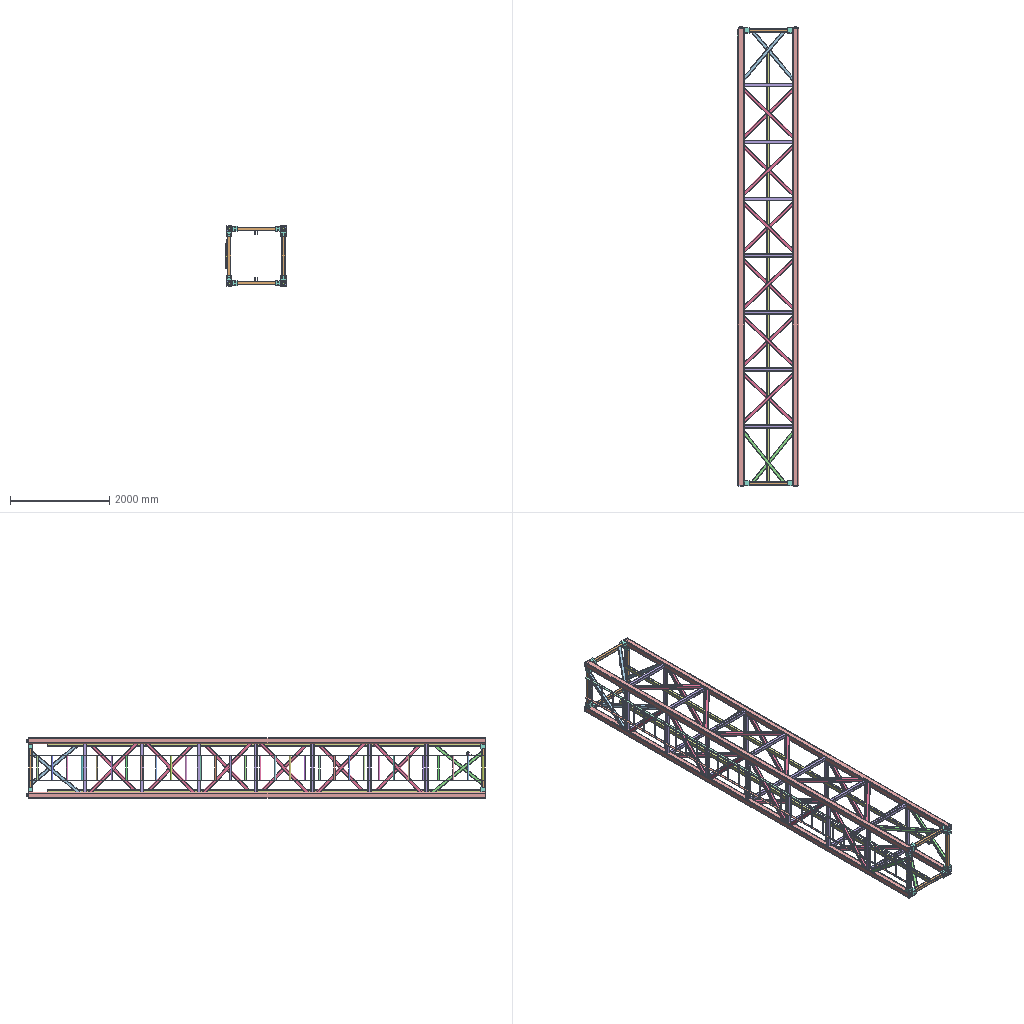Assembly | SolidWorks | 13 different items | 107 placed | box 1235 x 9290 x 1220 mm
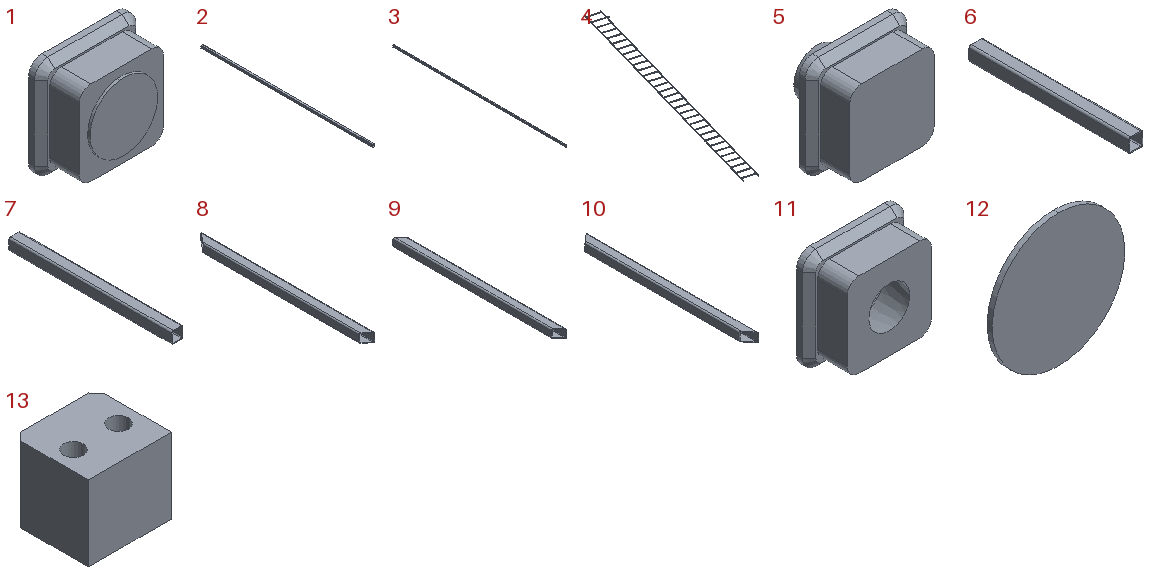Parts list (item | name | quantity | parent item | size | volume | features):
1 | (subassembly) | x4 | - | 120 x 53 x 120 mm | 407856 mm3 | -
2 | - | x4 | - | 120 x 9220 x 120 mm | 38826807 mm3 | features WeldMemberFeat 1, WeldmentFeature 1
3 | - | x2 | - | 60 x 8850 x 80 mm | 10935232 mm3 | features WeldMemberFeat 1, WeldmentFeature 1
4 | - | x1 | - | 3019 x 8991 x 40 mm | 7846988 mm3 | features WeldMemberFeat 2, Chamfer 1, LPattern 1, Sweep 1, WeldCornerFeat 1, WeldmentFeature 1
5 | - | x4 | - | 120 x 90 x 120 mm | 672208 mm3 | features Chamfer 2, ICE 2, Revolution 1
6 | - | x8 | - | 70 x 780 x 70 mm | 963783 mm3 | features WeldMemberFeat 1, WeldmentFeature 1
7 | - | x28 | - | 70 x 980 x 70 mm | 1210907 mm3 | features WeldMemberFeat 1, WeldmentFeature 1
8 | - | x4 | - | 70 x 1340 x 70 mm | 1567074 mm3 | features ICE 1, WeldMemberFeat 1, WeldmentFeature 1
9 | - | x24 | - | 70 x 1421 x 70 mm | 1672765 mm3 | features ICE 1, WeldMemberFeat 1, WeldmentFeature 1
10 | - | x4 | - | 70 x 1302 x 70 mm | 1520953 mm3 | features ICE 1, WeldMemberFeat 1, WeldmentFeature 1
11 | - | x4 | in 1 | 120 x 50 x 120 mm | 392776 mm3 | features Chamfer 1, Extrusion 1, ICE 1, RevCut 1
12 | - | x4 | in 1 | 80 x 3 x 80 mm | 15080 mm3 | features Extrusion 1
13 | - | x16 | - | 110 x 100 x 100 mm | 983814 mm3 | features Chamfer 1, Extrusion 1, HoleWzd 1
Mates (type | each side: item.copy, entity, surface, feature):
In the top assembly
Symmetric | 2.1 face plane Cold-formed hollow square steel (GB/T 6728-2002) 120×120×10(1) | 2.2 face plane Cold-formed hollow square steel (GB/T 6728-2002) 120×120×10(1) | assembly plane
DistanceDim | assembly plane | 2.1 face plane Cold-formed hollow square steel (GB/T 6728-2002) 120×120×10(1)
Coincident | 2.3 face plane Cold-formed hollow square steel (GB/T 6728-2002) 120×120×10(1) | assembly plane
Coincident | 2.1 face plane Cold-formed hollow square steel (GB/T 6728-2002) 120×120×10(1) | 11.1 face plane Boss-Extrude1
Width | 11.1 face plane Boss-Extrude2 | 11.1 face plane Boss-Extrude2 | 2.1 face plane Cold-formed hollow square steel (GB/T 6728-2002) 120×120×10(1) | 2.1 face plane Cold-formed hollow square steel (GB/T 6728-2002) 120×120×10(1)
Width | 2.1 face plane Cold-formed hollow square steel (GB/T 6728-2002) 120×120×10(1) | 2.1 face plane Cold-formed hollow square steel (GB/T 6728-2002) 120×120×10(1) | 11.1 face plane Boss-Extrude1 | 11.1 face plane Boss-Extrude1
Coincident | 2.1 face plane Cold-formed hollow square steel (GB/T 6728-2002) 120×120×10(1) | 5.1 face plane Boss-Extrude1
Width | 2.1 face plane Cold-formed hollow square steel (GB/T 6728-2002) 120×120×10(1) | 2.1 face plane Cold-formed hollow square steel (GB/T 6728-2002) 120×120×10(1) | 5.1 face plane Boss-Extrude1 | 5.1 face plane Boss-Extrude1 | 2 times
Coincident | 13.1 face plane Boss-Extrude1 | 11.2 face plane Boss-Extrude1
Width | 13.1 face plane Boss-Extrude1 | 13.1 face plane Boss-Extrude1 | 2.3 face plane Cold-formed hollow square steel (GB/T 6728-2002) 120×120×10(1) | 2.3 face plane Cold-formed hollow square steel (GB/T 6728-2002) 120×120×10(1)
Coincident | 13.1 face plane Boss-Extrude1 | 2.3 face plane Cold-formed hollow square steel (GB/T 6728-2002) 120×120×10(1)
Coincident | 2.3 face plane Cold-formed hollow square steel (GB/T 6728-2002) 120×120×10(1) | 13.2 face plane Boss-Extrude1
Coincident | 13.1 face plane Boss-Extrude1 | 13.2 face plane Boss-Extrude1
Width | 13.2 face plane Boss-Extrude1 | 13.2 face plane Boss-Extrude1 | 2.3 face plane Cold-formed hollow square steel (GB/T 6728-2002) 120×120×10(1) | 2.3 face plane Cold-formed hollow square steel (GB/T 6728-2002) 120×120×10(1)
Coincident | 13.3 face plane Boss-Extrude1 | 13.4 face plane Boss-Extrude1
Coincident | 13.1 face plane Boss-Extrude1 | 13.4 face plane Boss-Extrude1 | 2 times
Coincident | 13.2 face plane Boss-Extrude1 | 13.3 face plane Boss-Extrude1 | 2 times
Coincident | 5.2 face plane Boss-Extrude1 | 13.3 face plane Boss-Extrude1
Coincident | 6.1 face plane 19 (WeldMemberFeat) (+4 more in 5 files) Cold-formed hollow square steel (GB/T 6728-2002) 70×70×5(1) | 6.2 face plane 19 (WeldMemberFeat) (+4 more in 5 files) Cold-formed hollow square steel (GB/T 6728-2002) 70×70×5(1) | 2 times
Width | 6.2 face plane 19 (WeldMemberFeat) (+4 more in 5 files) Cold-formed hollow square steel (GB/T 6728-2002) 70×70×5(1) | 6.2 face plane 19 (WeldMemberFeat) (+4 more in 5 files) Cold-formed hollow square steel (GB/T 6728-2002) 70×70×5(1) | 13.5 face plane Boss-Extrude1 | 13.5 face plane Boss-Extrude1
Coincident | 13.1 face plane Boss-Extrude1 | 6.1 face plane 19 (WeldMemberFeat) (+4 more in 5 files) Cold-formed hollow square steel (GB/T 6728-2002) 70×70×5(1)
Width | 6.1 face plane 19 (WeldMemberFeat) (+4 more in 5 files) Cold-formed hollow square steel (GB/T 6728-2002) 70×70×5(1) | 6.1 face plane 19 (WeldMemberFeat) (+4 more in 5 files) Cold-formed hollow square steel (GB/T 6728-2002) 70×70×5(1) | 13.1 face plane Boss-Extrude1 | 13.1 face plane Boss-Extrude1
Width | 13.1 face plane Boss-Extrude1 | 13.1 face plane Boss-Extrude1 | 6.1 face plane 19 (WeldMemberFeat) (+4 more in 5 files) Cold-formed hollow square steel (GB/T 6728-2002) 70×70×5(1) | 6.1 face plane 19 (WeldMemberFeat) (+4 more in 5 files) Cold-formed hollow square steel (GB/T 6728-2002) 70×70×5(1)
Coincident | 6.3 face plane 19 (WeldMemberFeat) (+4 more in 5 files) Cold-formed hollow square steel (GB/T 6728-2002) 70×70×5(1) | 6.4 face plane 19 (WeldMemberFeat) (+4 more in 5 files) Cold-formed hollow square steel (GB/T 6728-2002) 70×70×5(1) | 2 times
Coincident | 13.2 face plane Boss-Extrude1 | 6.3 face plane 19 (WeldMemberFeat) (+4 more in 5 files) Cold-formed hollow square steel (GB/T 6728-2002) 70×70×5(1)
Width | 6.3 face plane 19 (WeldMemberFeat) (+4 more in 5 files) Cold-formed hollow square steel (GB/T 6728-2002) 70×70×5(1) | 6.3 face plane 19 (WeldMemberFeat) (+4 more in 5 files) Cold-formed hollow square steel (GB/T 6728-2002) 70×70×5(1) | 13.2 face plane Boss-Extrude1 | 13.2 face plane Boss-Extrude1 | 2 times
Width | 6.4 face plane 19 (WeldMemberFeat) (+4 more in 5 files) Cold-formed hollow square steel (GB/T 6728-2002) 70×70×5(1) | 6.4 face plane 19 (WeldMemberFeat) (+4 more in 5 files) Cold-formed hollow square steel (GB/T 6728-2002) 70×70×5(1) | 13.3 face plane Boss-Extrude1 | 13.3 face plane Boss-Extrude1
Width | 7.1 face plane 19 (WeldMemberFeat) (+4 more in 5 files) Cold-formed hollow square steel (GB/T 6728-2002) 70×70×5(1) | 7.1 face plane 19 (WeldMemberFeat) (+4 more in 5 files) Cold-formed hollow square steel (GB/T 6728-2002) 70×70×5(1) | 2.4 face plane Cold-formed hollow square steel (GB/T 6728-2002) 120×120×10(1) | 2.4 face plane Cold-formed hollow square steel (GB/T 6728-2002) 120×120×10(1)
Coincident | 7.1 face plane 19 (WeldMemberFeat) (+4 more in 5 files) Cold-formed hollow square steel (GB/T 6728-2002) 70×70×5(1) | 2.4 face plane Cold-formed hollow square steel (GB/T 6728-2002) 120×120×10(1)
DistanceDim | 11.2 face plane Boss-Extrude1 | 7.1 face plane 19 (WeldMemberFeat) (+4 more in 5 files) Cold-formed hollow square steel (GB/T 6728-2002) 70×70×5(1)
Coincident | 9.1 face plane Cut-Extrude1 | 2.4 face plane Cold-formed hollow square steel (GB/T 6728-2002) 120×120×10(1)
Coincident | 2.3 face plane Cold-formed hollow square steel (GB/T 6728-2002) 120×120×10(1) | 9.2 face plane Cut-Extrude1
DistanceDim | 9.2 edge | 7.2 face plane 19 (WeldMemberFeat) (+4 more in 5 files) Cold-formed hollow square steel (GB/T 6728-2002) 70×70×5(1)
Coincident | 2.1 face plane Cold-formed hollow square steel (GB/T 6728-2002) 120×120×10(1) | 9.3 face plane Cut-Extrude1
DistanceDim | 9.3 edge | 7.3 face plane 19 (WeldMemberFeat) (+4 more in 5 files) Cold-formed hollow square steel (GB/T 6728-2002) 70×70×5(1)
Coincident | 9.3 face plane 19 (WeldMemberFeat) (+4 more in 5 files) Cold-formed hollow square steel (GB/T 6728-2002) 70×70×5(1) | 9.4 face plane 19 (WeldMemberFeat) (+4 more in 5 files) Cold-formed hollow square steel (GB/T 6728-2002) 70×70×5(1)
Coincident | 2.2 face plane Cold-formed hollow square steel (GB/T 6728-2002) 120×120×10(1) | 9.4 face plane Cut-Extrude1
DistanceDim | 9.4 edge | 7.4 face plane 19 (WeldMemberFeat) (+4 more in 5 files) Cold-formed hollow square steel (GB/T 6728-2002) 70×70×5(1)
Coincident | 6.2 face plane 19 (WeldMemberFeat) (+4 more in 5 files) Cold-formed hollow square steel (GB/T 6728-2002) 70×70×5(1) | 10.1 face plane Cut-Extrude1
Coincident | 6.2 face plane 19 (WeldMemberFeat) (+4 more in 5 files) Cold-formed hollow square steel (GB/T 6728-2002) 70×70×5(1) | 10.1 face plane 19 (WeldMemberFeat) (+4 more in 5 files) Cold-formed hollow square steel (GB/T 6728-2002) 70×70×5(1)
Coincident | 2.3 face plane Cold-formed hollow square steel (GB/T 6728-2002) 120×120×10(1) | 10.1 face plane Cut-Extrude1
Coincident | 2.2 face plane Cold-formed hollow square steel (GB/T 6728-2002) 120×120×10(1) | 10.2 face plane Cut-Extrude1
Coincident | assembly face | 10.2 face plane 19 (WeldMemberFeat) (+4 more in 5 files) Cold-formed hollow square steel (GB/T 6728-2002) 70×70×5(1)
Coincident | 6.5 face plane 19 (WeldMemberFeat) (+4 more in 5 files) Cold-formed hollow square steel (GB/T 6728-2002) 70×70×5(1) | 10.2 face plane Cut-Extrude1
Coincident | 7.1 face plane 19 (WeldMemberFeat) (+4 more in 5 files) Cold-formed hollow square steel (GB/T 6728-2002) 70×70×5(1) | 7.5 face plane 19 (WeldMemberFeat) (+4 more in 5 files) Cold-formed hollow square steel (GB/T 6728-2002) 70×70×5(1)
Coincident | 2.3 face plane Cold-formed hollow square steel (GB/T 6728-2002) 120×120×10(1) | 7.5 face plane 19 (WeldMemberFeat) (+4 more in 5 files) Cold-formed hollow square steel (GB/T 6728-2002) 70×70×5(1)
Width | 7.5 face plane 19 (WeldMemberFeat) (+4 more in 5 files) Cold-formed hollow square steel (GB/T 6728-2002) 70×70×5(1) | 7.5 face plane 19 (WeldMemberFeat) (+4 more in 5 files) Cold-formed hollow square steel (GB/T 6728-2002) 70×70×5(1) | 2.3 face plane Cold-formed hollow square steel (GB/T 6728-2002) 120×120×10(1) | 2.3 face plane Cold-formed hollow square steel (GB/T 6728-2002) 120×120×10(1)
Coincident | 7.5 face plane 19 (WeldMemberFeat) (+4 more in 5 files) Cold-formed hollow square steel (GB/T 6728-2002) 70×70×5(1) | 7.6 face plane 19 (WeldMemberFeat) (+4 more in 5 files) Cold-formed hollow square steel (GB/T 6728-2002) 70×70×5(1) | 2 times
Width | 7.6 face plane 19 (WeldMemberFeat) (+4 more in 5 files) Cold-formed hollow square steel (GB/T 6728-2002) 70×70×5(1) | 7.6 face plane 19 (WeldMemberFeat) (+4 more in 5 files) Cold-formed hollow square steel (GB/T 6728-2002) 70×70×5(1) | 2.2 face plane Cold-formed hollow square steel (GB/T 6728-2002) 120×120×10(1) | 2.2 face plane Cold-formed hollow square steel (GB/T 6728-2002) 120×120×10(1)
Coincident | 4.1 face plane GB/T 704-1988 hot-rolled flat steel 40×6(1) | 6.4 face plane 19 (WeldMemberFeat) (+4 more in 5 files) Cold-formed hollow square steel (GB/T 6728-2002) 70×70×5(1)
Width | 2.3 face plane Cold-formed hollow square steel (GB/T 6728-2002) 120×120×10(1) | 2.1 face plane Cold-formed hollow square steel (GB/T 6728-2002) 120×120×10(1) | 4.1 face plane GB/T 704-1988 hot-rolled flat steel 40×6(1) | 4.1 face plane GB/T 704-1988 hot-rolled flat steel 40×6(1)
Coincident | 4.1 face plane GB/T 704-1988 hot-rolled flat steel 40×6(1) | 11.2 face plane Boss-Extrude1
Coincident | 6.2 face plane 19 (WeldMemberFeat) (+4 more in 5 files) Cold-formed hollow square steel (GB/T 6728-2002) 70×70×5(1) | 3.1 face plane Cold-formed hollow rectangular steel (GB/T 6728-2002) 80×60×5(1)
Coincident | 3.1 plane | assembly plane
Coincident | 8.1 face plane Cut-Extrude1 | 6.1 face plane 19 (WeldMemberFeat) (+4 more in 5 files) Cold-formed hollow square steel (GB/T 6728-2002) 70×70×5(1)
Coincident | 8.1 face plane Cut-Extrude1 | 2.4 face plane Cold-formed hollow square steel (GB/T 6728-2002) 120×120×10(1)
Coincident | 6.6 face plane 19 (WeldMemberFeat) (+4 more in 5 files) Cold-formed hollow square steel (GB/T 6728-2002) 70×70×5(1) | 8.2 face plane Cut-Extrude1
Coincident | 2.1 face plane Cold-formed hollow square steel (GB/T 6728-2002) 120×120×10(1) | 8.2 face plane Cut-Extrude1
Coincident | 6.3 face plane 19 (WeldMemberFeat) (+4 more in 5 files) Cold-formed hollow square steel (GB/T 6728-2002) 70×70×5(1) | 8.3 face plane Cut-Extrude1
Coincident | 2.3 face plane Cold-formed hollow square steel (GB/T 6728-2002) 120×120×10(1) | 8.3 face plane Cut-Extrude1
Coincident | 6.7 face plane 19 (WeldMemberFeat) (+4 more in 5 files) Cold-formed hollow square steel (GB/T 6728-2002) 70×70×5(1) | 8.4 face plane Cut-Extrude1
Coincident | 2.2 face plane Cold-formed hollow square steel (GB/T 6728-2002) 120×120×10(1) | 8.4 face plane Cut-Extrude1
Coincident | 2.1 face plane Cold-formed hollow square steel (GB/T 6728-2002) 120×120×10(1) | 10.3 face plane Cut-Extrude1
Coincident | assembly face | 10.3 face plane 19 (WeldMemberFeat) (+4 more in 5 files) Cold-formed hollow square steel (GB/T 6728-2002) 70×70×5(1)
Coincident | 6.4 face plane 19 (WeldMemberFeat) (+4 more in 5 files) Cold-formed hollow square steel (GB/T 6728-2002) 70×70×5(1) | 10.3 face plane Cut-Extrude1
Coincident | 6.8 face plane 19 (WeldMemberFeat) (+4 more in 5 files) Cold-formed hollow square steel (GB/T 6728-2002) 70×70×5(1) | 10.4 face plane Cut-Extrude1
Coincident | assembly face | 10.4 face plane 19 (WeldMemberFeat) (+4 more in 5 files) Cold-formed hollow square steel (GB/T 6728-2002) 70×70×5(1)
Coincident | 2.4 face plane Cold-formed hollow square steel (GB/T 6728-2002) 120×120×10(1) | 10.4 face plane Cut-Extrude1
Coincident | 2.1 face plane Cold-formed hollow square steel (GB/T 6728-2002) 120×120×10(1) | 9.5 face plane Cut-Extrude1
Coincident | 2.4 face plane Cold-formed hollow square steel (GB/T 6728-2002) 120×120×10(1) | 9.6 face plane Cut-Extrude1
DistanceDim | 9.5 edge | 7.5 face plane 19 (WeldMemberFeat) (+4 more in 5 files) Cold-formed hollow square steel (GB/T 6728-2002) 70×70×5(1)
DistanceDim | 9.6 edge | 7.6 face plane 19 (WeldMemberFeat) (+4 more in 5 files) Cold-formed hollow square steel (GB/T 6728-2002) 70×70×5(1)
Coincident | 2.3 face plane Cold-formed hollow square steel (GB/T 6728-2002) 120×120×10(1) | 9.7 face plane Cut-Extrude1
DistanceDim | 7.7 face plane 19 (WeldMemberFeat) (+4 more in 5 files) Cold-formed hollow square steel (GB/T 6728-2002) 70×70×5(1) | 9.7 edge
Coincident | 8.2 face plane 19 (WeldMemberFeat) (+4 more in 5 files) Cold-formed hollow square steel (GB/T 6728-2002) 70×70×5(1) | 6.1 face plane 19 (WeldMemberFeat) (+4 more in 5 files) Cold-formed hollow square steel (GB/T 6728-2002) 70×70×5(1)
Coincident | 8.1 face plane 19 (WeldMemberFeat) (+4 more in 5 files) Cold-formed hollow square steel (GB/T 6728-2002) 70×70×5(1) | 6.6 face plane 19 (WeldMemberFeat) (+4 more in 5 files) Cold-formed hollow square steel (GB/T 6728-2002) 70×70×5(1)
Coincident | 9.3 face plane 19 (WeldMemberFeat) (+4 more in 5 files) Cold-formed hollow square steel (GB/T 6728-2002) 70×70×5(1) | 7.1 face plane 19 (WeldMemberFeat) (+4 more in 5 files) Cold-formed hollow square steel (GB/T 6728-2002) 70×70×5(1)
Coincident | 9.1 face plane 19 (WeldMemberFeat) (+4 more in 5 files) Cold-formed hollow square steel (GB/T 6728-2002) 70×70×5(1) | 7.3 face plane 19 (WeldMemberFeat) (+4 more in 5 files) Cold-formed hollow square steel (GB/T 6728-2002) 70×70×5(1)
Coincident | 9.2 face plane 19 (WeldMemberFeat) (+4 more in 5 files) Cold-formed hollow square steel (GB/T 6728-2002) 70×70×5(1) | 7.4 face plane 19 (WeldMemberFeat) (+4 more in 5 files) Cold-formed hollow square steel (GB/T 6728-2002) 70×70×5(1)
Coincident | 2.4 face plane Cold-formed hollow square steel (GB/T 6728-2002) 120×120×10(1) | 9.8 face plane Cut-Extrude1
DistanceDim | 9.8 edge | 7.8 face plane 19 (WeldMemberFeat) (+4 more in 5 files) Cold-formed hollow square steel (GB/T 6728-2002) 70×70×5(1)
DistanceDim | 9.1 edge | 7.3 face plane 19 (WeldMemberFeat) (+4 more in 5 files) Cold-formed hollow square steel (GB/T 6728-2002) 70×70×5(1)
Coincident | 3.1 face plane Cold-formed hollow rectangular steel (GB/T 6728-2002) 80×60×5(1) | 11.2 face plane Boss-Extrude1
Coincident | 8.4 face plane 19 (WeldMemberFeat) (+4 more in 5 files) Cold-formed hollow square steel (GB/T 6728-2002) 70×70×5(1) | 6.3 face plane 19 (WeldMemberFeat) (+4 more in 5 files) Cold-formed hollow square steel (GB/T 6728-2002) 70×70×5(1)
Coincident | 8.3 face plane 19 (WeldMemberFeat) (+4 more in 5 files) Cold-formed hollow square steel (GB/T 6728-2002) 70×70×5(1) | 6.7 face plane 19 (WeldMemberFeat) (+4 more in 5 files) Cold-formed hollow square steel (GB/T 6728-2002) 70×70×5(1)
Coincident | 7.5 face plane 19 (WeldMemberFeat) (+4 more in 5 files) Cold-formed hollow square steel (GB/T 6728-2002) 70×70×5(1) | 9.6 face plane 19 (WeldMemberFeat) (+4 more in 5 files) Cold-formed hollow square steel (GB/T 6728-2002) 70×70×5(1)
Coincident | 7.6 face plane 19 (WeldMemberFeat) (+4 more in 5 files) Cold-formed hollow square steel (GB/T 6728-2002) 70×70×5(1) | 9.5 face plane 19 (WeldMemberFeat) (+4 more in 5 files) Cold-formed hollow square steel (GB/T 6728-2002) 70×70×5(1)
Coincident | 7.7 face plane 19 (WeldMemberFeat) (+4 more in 5 files) Cold-formed hollow square steel (GB/T 6728-2002) 70×70×5(1) | 9.8 face plane 19 (WeldMemberFeat) (+4 more in 5 files) Cold-formed hollow square steel (GB/T 6728-2002) 70×70×5(1)
Coincident | 7.8 face plane 19 (WeldMemberFeat) (+4 more in 5 files) Cold-formed hollow square steel (GB/T 6728-2002) 70×70×5(1) | 9.7 face plane 19 (WeldMemberFeat) (+4 more in 5 files) Cold-formed hollow square steel (GB/T 6728-2002) 70×70×5(1)
In subassembly 1
Concentric | 11.3 face cylinder Cut-Revolve1 | 12.1 face cylinder Boss-Extrude1
Coincident | 11.3 face plane Boss-Extrude2 | 12.1 face plane Boss-Extrude1